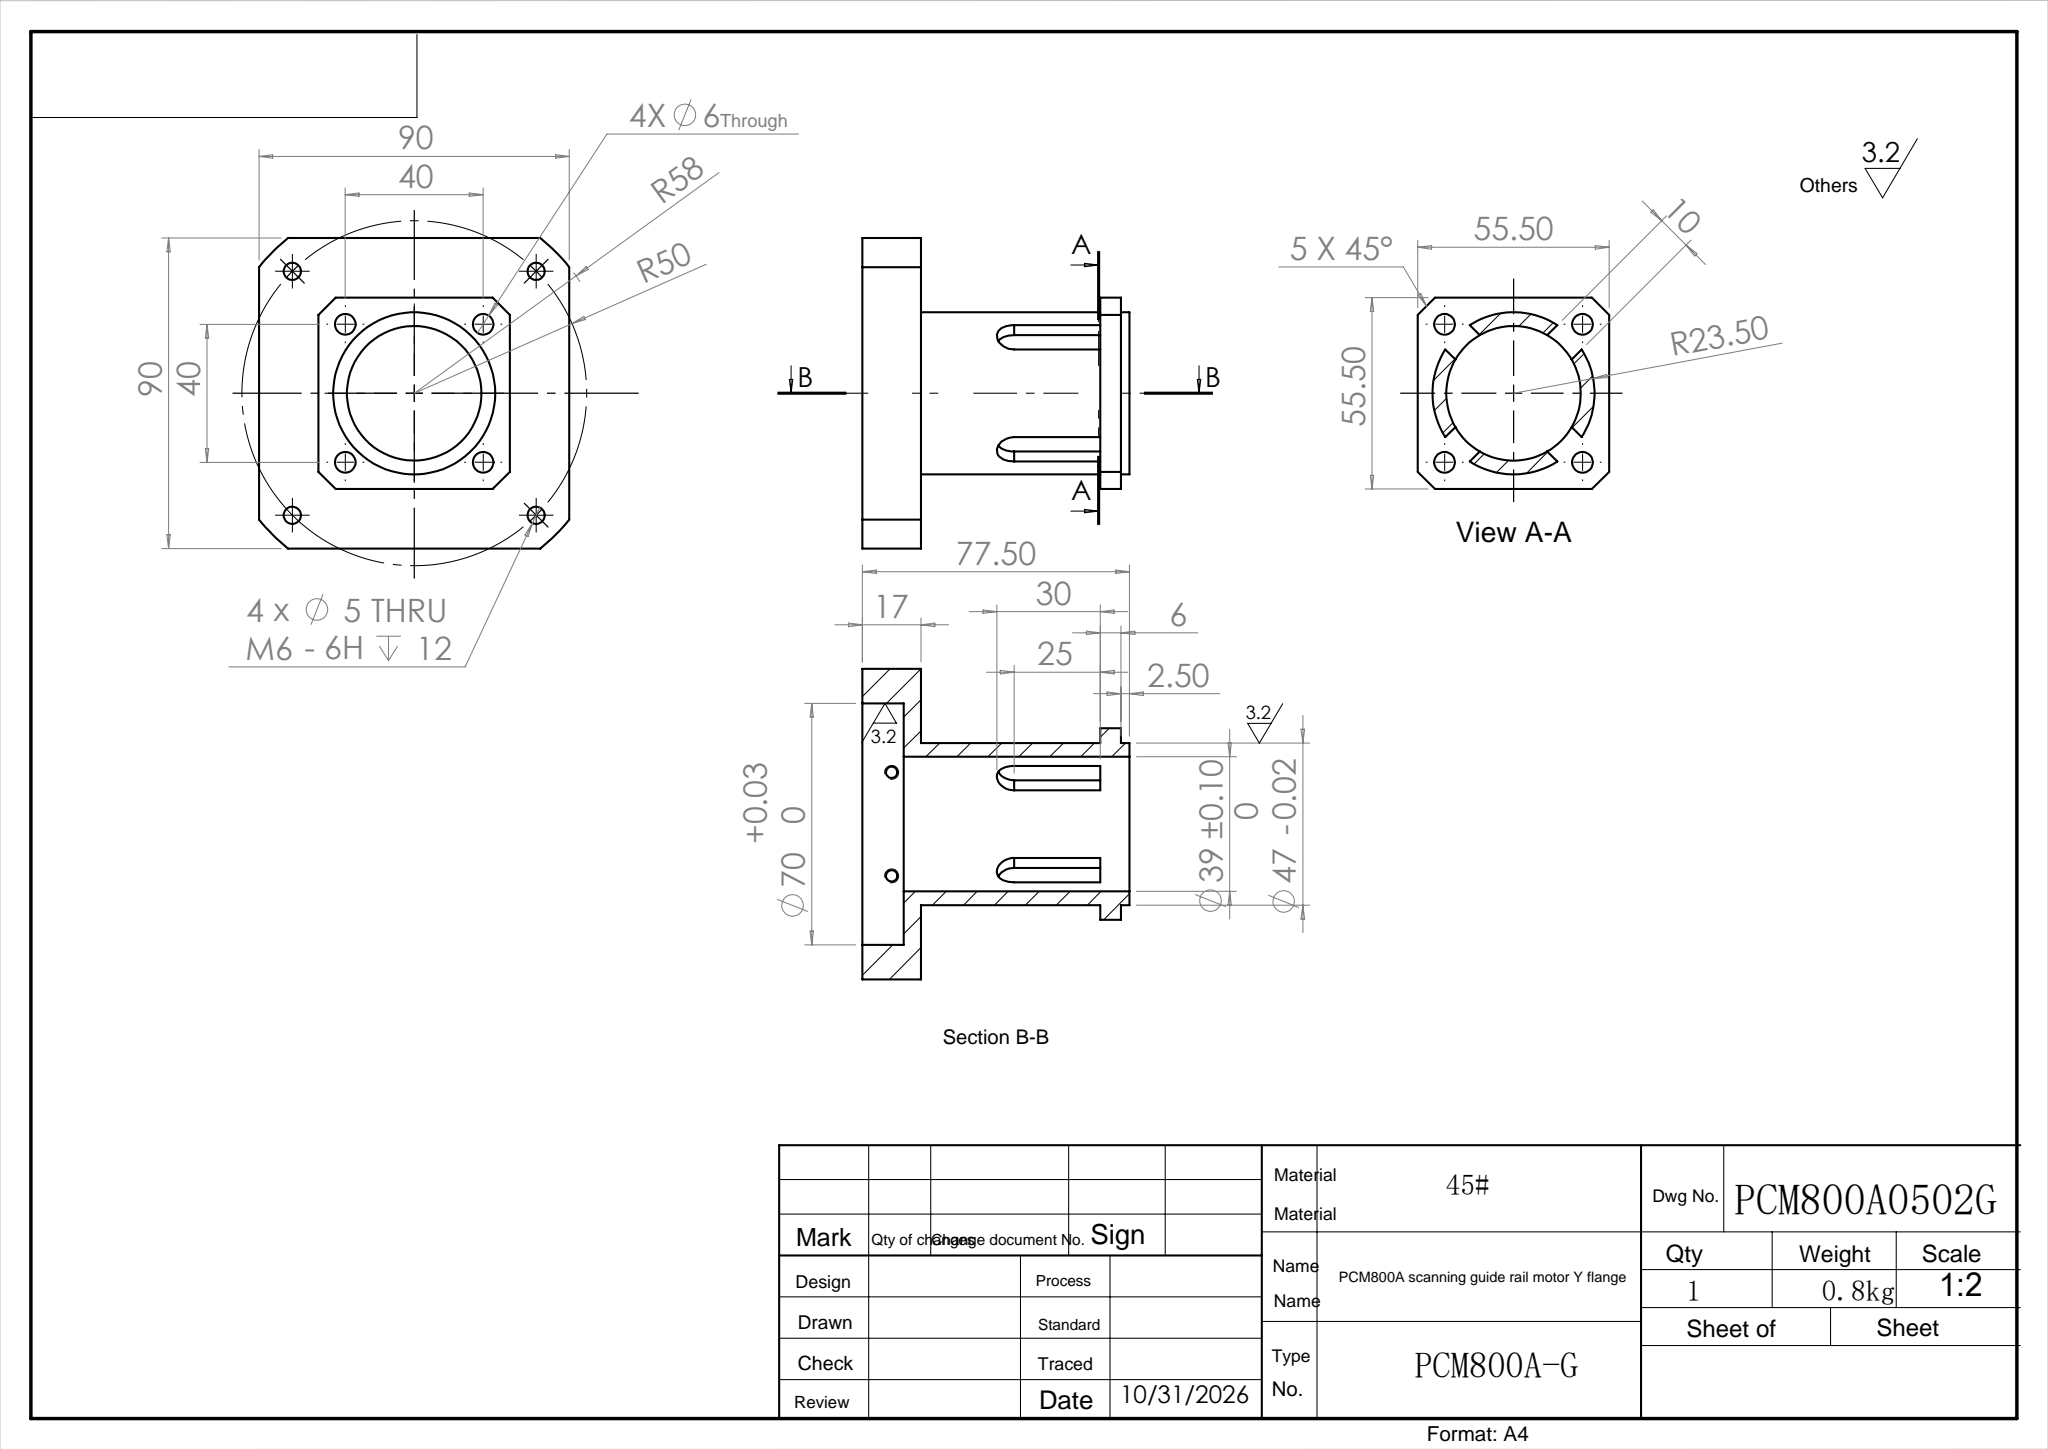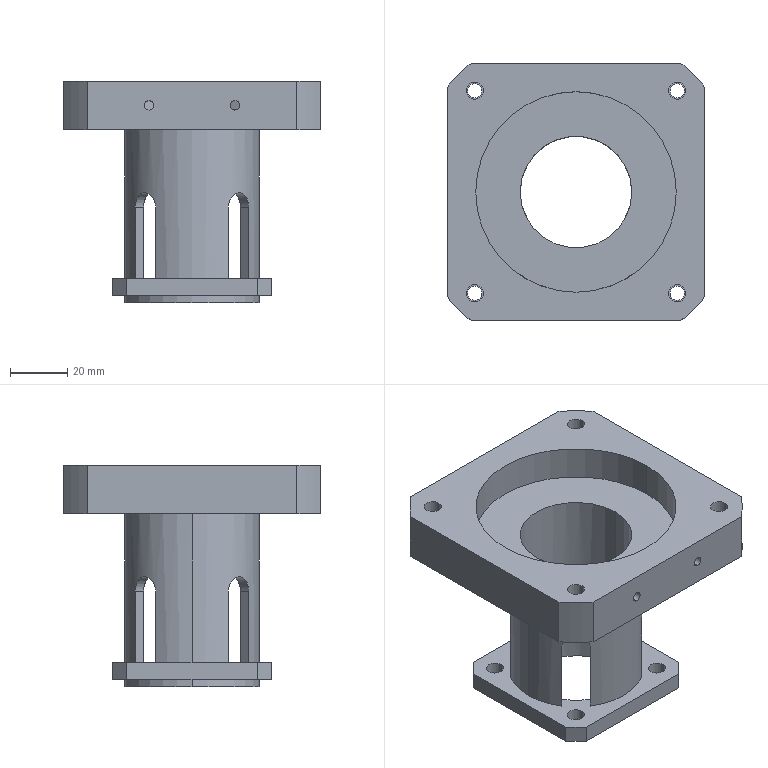Part | SolidWorks | features Cut 6, Boss 3, HoleWzd 2, 3DProfileFeature 1, Chamfer 1, Extrusion 1 | 1 solid | 74 faces | box 90 x 90 x 77.5 mm | volume 116443 mm3 | cylinder 44 | plane 30 | commonest cylinder face diameters 6 x16 5 x8 3.3 x4 10 x4 47 x4 116 x4